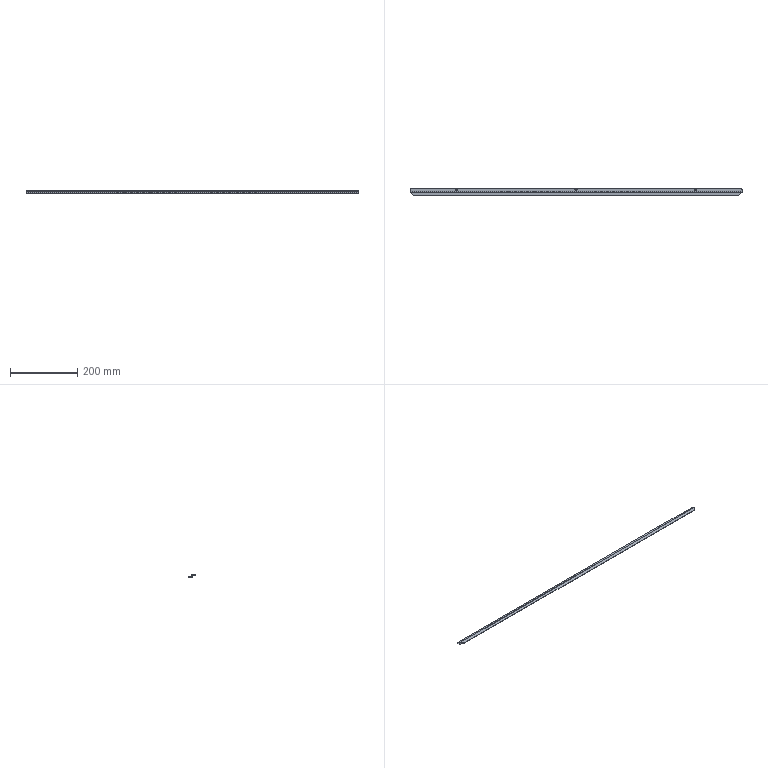Part | SolidWorks | features Chamfer 1, Fillet 1, FlatPattern 1, HoleWzd 1, SMBaseFlange 1, SheetMetal 1 | 1 solid | 30 faces | box 986 x 22 x 8.2 mm | volume 33274 mm3 | plane 18 | cylinder 12 | commonest cylinder face diameters 6 x8 0.4 x2 2.8 x2
STEP:
#1=CARTESIAN_POINT('',(-350.5,-5.,0.));
#2=VERTEX_POINT('',#1);
#3=CARTESIAN_POINT('',(-356.5,-5.,0.));
#4=VERTEX_POINT('',#3);
#5=CARTESIAN_POINT('',(-353.5,-5.,0.));
#6=DIRECTION('',(0.,0.,-1.));
#7=DIRECTION('',(0.,1.,0.));
#8=AXIS2_PLACEMENT_3D('',#5,#6,#7);
#9=CIRCLE('',#8,3.);
#10=EDGE_CURVE('',#2,#4,#9,.T.);
#11=ORIENTED_EDGE('',*,*,#10,.T.);
#12=CARTESIAN_POINT('',(-356.5,-5.,1.2));
#13=VERTEX_POINT('',#12);
#14=CARTESIAN_POINT('',(-356.5,-5.,1.2));
#15=DIRECTION('',(0.,0.,1.));
#16=VECTOR('',#15,1000.);
#17=LINE('',#14,#16);
#18=EDGE_CURVE('',#4,#13,#17,.T.);
#19=ORIENTED_EDGE('',*,*,#18,.T.);
#20=CARTESIAN_POINT('',(-350.5,-5.,1.2));
#21=VERTEX_POINT('',#20);
#22=CARTESIAN_POINT('',(-353.5,-5.,1.2));
#23=DIRECTION('',(0.,0.,1.));
#24=DIRECTION('',(1.,0.,0.));
#25=AXIS2_PLACEMENT_3D('',#22,#23,#24);
#26=CIRCLE('',#25,3.);
#27=EDGE_CURVE('',#13,#21,#26,.T.);
#28=ORIENTED_EDGE('',*,*,#27,.T.);
#29=CARTESIAN_POINT('',(-350.5,-5.,1.2));
#30=DIRECTION('',(0.,0.,1.));
#31=VECTOR('',#30,1000.);
#32=LINE('',#29,#31);
#33=EDGE_CURVE('',#2,#21,#32,.T.);
#34=ORIENTED_EDGE('',*,*,#33,.F.);
#35=EDGE_LOOP('',(#11,#19,#28,#34));
#36=FACE_OUTER_BOUND('',#35,.T.);
#37=CARTESIAN_POINT('',(-353.5,-5.,1.2));
#38=DIRECTION('',(0.,0.,1.));
#39=DIRECTION('',(1.,0.,0.));
#40=AXIS2_PLACEMENT_3D('',#37,#38,#39);
#41=CYLINDRICAL_SURFACE('',#40,3.);
#42=ADVANCED_FACE('',(#36),#41,.F.);
#43=CARTESIAN_POINT('',(3.,-5.,0.));
#44=VERTEX_POINT('',#43);
#45=CARTESIAN_POINT('',(-3.,-5.,0.));
#46=VERTEX_POINT('',#45);
#47=CARTESIAN_POINT('',(0.,-5.,0.));
#48=DIRECTION('',(0.,0.,-1.));
#49=DIRECTION('',(0.,1.,0.));
#50=AXIS2_PLACEMENT_3D('',#47,#48,#49);
#51=CIRCLE('',#50,3.);
#52=EDGE_CURVE('',#44,#46,#51,.T.);
#53=ORIENTED_EDGE('',*,*,#52,.T.);
#54=CARTESIAN_POINT('',(-3.,-5.,1.2));
#55=VERTEX_POINT('',#54);
#56=CARTESIAN_POINT('',(-3.,-5.,1.2));
#57=DIRECTION('',(0.,0.,1.));
#58=VECTOR('',#57,1000.);
#59=LINE('',#56,#58);
#60=EDGE_CURVE('',#46,#55,#59,.T.);
#61=ORIENTED_EDGE('',*,*,#60,.T.);
#62=CARTESIAN_POINT('',(3.,-5.,1.2));
#63=VERTEX_POINT('',#62);
#64=CARTESIAN_POINT('',(0.,-5.,1.2));
#65=DIRECTION('',(0.,0.,1.));
#66=DIRECTION('',(1.,0.,0.));
#67=AXIS2_PLACEMENT_3D('',#64,#65,#66);
#68=CIRCLE('',#67,3.);
#69=EDGE_CURVE('',#55,#63,#68,.T.);
#70=ORIENTED_EDGE('',*,*,#69,.T.);
#71=CARTESIAN_POINT('',(3.,-5.,1.2));
#72=DIRECTION('',(0.,0.,1.));
#73=VECTOR('',#72,1000.);
#74=LINE('',#71,#73);
#75=EDGE_CURVE('',#44,#63,#74,.T.);
#76=ORIENTED_EDGE('',*,*,#75,.F.);
#77=EDGE_LOOP('',(#53,#61,#70,#76));
#78=FACE_OUTER_BOUND('',#77,.T.);
#79=CARTESIAN_POINT('',(0.,-5.,1.2));
#80=DIRECTION('',(0.,0.,1.));
#81=DIRECTION('',(1.,0.,0.));
#82=AXIS2_PLACEMENT_3D('',#79,#80,#81);
#83=CYLINDRICAL_SURFACE('',#82,3.);
#84=ADVANCED_FACE('',(#78),#83,.F.);
#85=CARTESIAN_POINT('',(356.5,-5.,0.));
#86=VERTEX_POINT('',#85);
#87=CARTESIAN_POINT('',(350.5,-5.,0.));
#88=VERTEX_POINT('',#87);
#89=CARTESIAN_POINT('',(353.5,-5.,0.));
#90=DIRECTION('',(0.,0.,-1.));
#91=DIRECTION('',(0.,1.,0.));
#92=AXIS2_PLACEMENT_3D('',#89,#90,#91);
#93=CIRCLE('',#92,3.);
#94=EDGE_CURVE('',#86,#88,#93,.T.);
#95=ORIENTED_EDGE('',*,*,#94,.T.);
#96=CARTESIAN_POINT('',(350.5,-5.,1.2));
#97=VERTEX_POINT('',#96);
#98=CARTESIAN_POINT('',(350.5,-5.,1.2));
#99=DIRECTION('',(0.,0.,1.));
#100=VECTOR('',#99,1000.);
#101=LINE('',#98,#100);
#102=EDGE_CURVE('',#88,#97,#101,.T.);
#103=ORIENTED_EDGE('',*,*,#102,.T.);
#104=CARTESIAN_POINT('',(356.5,-5.,1.2));
#105=VERTEX_POINT('',#104);
#106=CARTESIAN_POINT('',(353.5,-5.,1.2));
#107=DIRECTION('',(0.,0.,1.));
#108=DIRECTION('',(1.,0.,0.));
#109=AXIS2_PLACEMENT_3D('',#106,#107,#108);
#110=CIRCLE('',#109,3.);
#111=EDGE_CURVE('',#97,#105,#110,.T.);
#112=ORIENTED_EDGE('',*,*,#111,.T.);
#113=CARTESIAN_POINT('',(356.5,-5.,1.2));
#114=DIRECTION('',(0.,0.,1.));
#115=VECTOR('',#114,1000.);
#116=LINE('',#113,#115);
#117=EDGE_CURVE('',#86,#105,#116,.T.);
#118=ORIENTED_EDGE('',*,*,#117,.F.);
#119=EDGE_LOOP('',(#95,#103,#112,#118));
#120=FACE_OUTER_BOUND('',#119,.T.);
#121=CARTESIAN_POINT('',(353.5,-5.,1.2));
#122=DIRECTION('',(0.,0.,1.));
#123=DIRECTION('',(1.,0.,0.));
#124=AXIS2_PLACEMENT_3D('',#121,#122,#123);
#125=CYLINDRICAL_SURFACE('',#124,3.);
#126=ADVANCED_FACE('',(#120),#125,.F.);
#127=CARTESIAN_POINT('',(-353.5,-5.,1.2));
#128=DIRECTION('',(0.,0.,1.));
#129=DIRECTION('',(1.,0.,0.));
#130=AXIS2_PLACEMENT_3D('',#127,#128,#129);
#131=CIRCLE('',#130,3.);
#132=EDGE_CURVE('',#21,#13,#131,.T.);
#133=ORIENTED_EDGE('',*,*,#132,.F.);
#134=ORIENTED_EDGE('',*,*,#27,.F.);
#135=EDGE_LOOP('',(#133,#134));
#136=FACE_BOUND('',#135,.T.);
#137=CARTESIAN_POINT('',(353.5,-5.,1.2));
#138=DIRECTION('',(0.,0.,1.));
#139=DIRECTION('',(1.,0.,0.));
#140=AXIS2_PLACEMENT_3D('',#137,#138,#139);
#141=CIRCLE('',#140,3.);
#142=EDGE_CURVE('',#105,#97,#141,.T.);
#143=ORIENTED_EDGE('',*,*,#142,.F.);
#144=ORIENTED_EDGE('',*,*,#111,.F.);
#145=EDGE_LOOP('',(#143,#144));
#146=FACE_BOUND('',#145,.T.);
#147=CARTESIAN_POINT('',(490.,0.,1.2));
#148=VERTEX_POINT('',#147);
#149=CARTESIAN_POINT('',(-490.,0.,1.2));
#150=VERTEX_POINT('',#149);
#151=CARTESIAN_POINT('',(493.,0.,1.2));
#152=DIRECTION('',(-1.,0.,0.));
#153=VECTOR('',#152,1000.);
#154=LINE('',#151,#153);
#155=EDGE_CURVE('',#148,#150,#154,.T.);
#156=ORIENTED_EDGE('',*,*,#155,.T.);
#157=CARTESIAN_POINT('',(-493.,-3.,1.2));
#158=VERTEX_POINT('',#157);
#159=CARTESIAN_POINT('',(-490.,-3.,1.2));
#160=DIRECTION('',(0.,0.,1.));
#161=DIRECTION('',(0.,1.,0.));
#162=AXIS2_PLACEMENT_3D('',#159,#160,#161);
#163=CIRCLE('',#162,3.);
#164=EDGE_CURVE('',#150,#158,#163,.T.);
#165=ORIENTED_EDGE('',*,*,#164,.T.);
#166=CARTESIAN_POINT('',(-493.,-10.6,1.2));
#167=VERTEX_POINT('',#166);
#168=CARTESIAN_POINT('',(-493.,0.,1.2));
#169=DIRECTION('',(0.,-1.,0.));
#170=VECTOR('',#169,1000.);
#171=LINE('',#168,#170);
#172=EDGE_CURVE('',#158,#167,#171,.T.);
#173=ORIENTED_EDGE('',*,*,#172,.T.);
#174=CARTESIAN_POINT('',(493.,-10.6,1.2));
#175=VERTEX_POINT('',#174);
#176=CARTESIAN_POINT('',(493.,-10.6,1.2));
#177=DIRECTION('',(-1.,0.,0.));
#178=VECTOR('',#177,1000.);
#179=LINE('',#176,#178);
#180=EDGE_CURVE('',#175,#167,#179,.T.);
#181=ORIENTED_EDGE('',*,*,#180,.F.);
#182=CARTESIAN_POINT('',(493.,-3.,1.2));
#183=VERTEX_POINT('',#182);
#184=CARTESIAN_POINT('',(493.,0.,1.2));
#185=DIRECTION('',(0.,-1.,0.));
#186=VECTOR('',#185,1000.);
#187=LINE('',#184,#186);
#188=EDGE_CURVE('',#183,#175,#187,.T.);
#189=ORIENTED_EDGE('',*,*,#188,.F.);
#190=CARTESIAN_POINT('',(490.,-3.,1.2));
#191=DIRECTION('',(0.,0.,1.));
#192=DIRECTION('',(0.,1.,0.));
#193=AXIS2_PLACEMENT_3D('',#190,#191,#192);
#194=CIRCLE('',#193,3.);
#195=EDGE_CURVE('',#183,#148,#194,.T.);
#196=ORIENTED_EDGE('',*,*,#195,.T.);
#197=EDGE_LOOP('',(#156,#165,#173,#181,#189,#196));
#198=FACE_OUTER_BOUND('',#197,.T.);
#199=CARTESIAN_POINT('',(0.,-5.,1.2));
#200=DIRECTION('',(0.,0.,1.));
#201=DIRECTION('',(1.,0.,0.));
#202=AXIS2_PLACEMENT_3D('',#199,#200,#201);
#203=CIRCLE('',#202,3.);
#204=EDGE_CURVE('',#63,#55,#203,.T.);
#205=ORIENTED_EDGE('',*,*,#204,.F.);
#206=ORIENTED_EDGE('',*,*,#69,.F.);
#207=EDGE_LOOP('',(#205,#206));
#208=FACE_BOUND('',#207,.T.);
#209=CARTESIAN_POINT('',(493.,0.,1.2));
#210=DIRECTION('',(0.,0.,-1.));
#211=DIRECTION('',(0.,1.,0.));
#212=AXIS2_PLACEMENT_3D('',#209,#210,#211);
#213=PLANE('',#212);
#214=ADVANCED_FACE('',(#136,#146,#198,#208),#213,.F.);
#215=CARTESIAN_POINT('',(493.,-12.,1.4));
#216=VERTEX_POINT('',#215);
#217=CARTESIAN_POINT('',(493.,-10.8,1.4));
#218=VERTEX_POINT('',#217);
#219=CARTESIAN_POINT('',(493.,-12.,1.4));
#220=DIRECTION('',(0.,1.,0.));
#221=VECTOR('',#220,1000.);
#222=LINE('',#219,#221);
#223=EDGE_CURVE('',#216,#218,#222,.T.);
#224=ORIENTED_EDGE('',*,*,#223,.F.);
#225=CARTESIAN_POINT('',(493.,-10.6,0.));
#226=VERTEX_POINT('',#225);
#227=CARTESIAN_POINT('',(493.,-10.6,1.4));
#228=DIRECTION('',(-1.,0.,0.));
#229=DIRECTION('',(0.,0.,-1.));
#230=AXIS2_PLACEMENT_3D('',#227,#228,#229);
#231=CIRCLE('',#230,1.4);
#232=EDGE_CURVE('',#226,#216,#231,.T.);
#233=ORIENTED_EDGE('',*,*,#232,.F.);
#234=CARTESIAN_POINT('',(493.,-10.6,1.2));
#235=DIRECTION('',(0.,0.,-1.));
#236=VECTOR('',#235,1000.);
#237=LINE('',#234,#236);
#238=EDGE_CURVE('',#175,#226,#237,.T.);
#239=ORIENTED_EDGE('',*,*,#238,.F.);
#240=CARTESIAN_POINT('',(493.,-10.6,1.4));
#241=DIRECTION('',(-1.,0.,0.));
#242=DIRECTION('',(0.,0.,-1.));
#243=AXIS2_PLACEMENT_3D('',#240,#241,#242);
#244=CIRCLE('',#243,0.2);
#245=EDGE_CURVE('',#175,#218,#244,.T.);
#246=ORIENTED_EDGE('',*,*,#245,.T.);
#247=EDGE_LOOP('',(#224,#233,#239,#246));
#248=FACE_OUTER_BOUND('',#247,.T.);
#249=CARTESIAN_POINT('',(493.,-12.,1.4));
#250=DIRECTION('',(1.,0.,0.));
#251=DIRECTION('',(0.,0.,-1.));
#252=AXIS2_PLACEMENT_3D('',#249,#250,#251);
#253=PLANE('',#252);
#254=ADVANCED_FACE('',(#248),#253,.T.);
#255=CARTESIAN_POINT('',(493.,-12.,6.8));
#256=VERTEX_POINT('',#255);
#257=CARTESIAN_POINT('',(493.,-12.,0.));
#258=DIRECTION('',(0.,0.,1.));
#259=VECTOR('',#258,1000.);
#260=LINE('',#257,#259);
#261=EDGE_CURVE('',#216,#256,#260,.T.);
#262=ORIENTED_EDGE('',*,*,#261,.F.);
#263=ORIENTED_EDGE('',*,*,#223,.T.);
#264=CARTESIAN_POINT('',(493.,-10.8,6.8));
#265=VERTEX_POINT('',#264);
#266=CARTESIAN_POINT('',(493.,-10.8,0.));
#267=DIRECTION('',(0.,0.,1.));
#268=VECTOR('',#267,1000.);
#269=LINE('',#266,#268);
#270=EDGE_CURVE('',#218,#265,#269,.T.);
#271=ORIENTED_EDGE('',*,*,#270,.T.);
#272=CARTESIAN_POINT('',(493.,-10.8,6.8));
#273=DIRECTION('',(0.,-1.,0.));
#274=VECTOR('',#273,1000.);
#275=LINE('',#272,#274);
#276=EDGE_CURVE('',#265,#256,#275,.T.);
#277=ORIENTED_EDGE('',*,*,#276,.T.);
#278=EDGE_LOOP('',(#262,#263,#271,#277));
#279=FACE_OUTER_BOUND('',#278,.T.);
#280=CARTESIAN_POINT('',(493.,-10.6,1.2));
#281=DIRECTION('',(1.,0.,0.));
#282=DIRECTION('',(0.,0.,-1.));
#283=AXIS2_PLACEMENT_3D('',#280,#281,#282);
#284=PLANE('',#283);
#285=ADVANCED_FACE('',(#279),#284,.T.);
#286=CARTESIAN_POINT('',(-493.,-10.6,0.));
#287=VERTEX_POINT('',#286);
#288=CARTESIAN_POINT('',(-493.,-10.6,0.));
#289=DIRECTION('',(0.,0.,1.));
#290=VECTOR('',#289,1000.);
#291=LINE('',#288,#290);
#292=EDGE_CURVE('',#287,#167,#291,.T.);
#293=ORIENTED_EDGE('',*,*,#292,.F.);
#294=CARTESIAN_POINT('',(-493.,-12.,1.4));
#295=VERTEX_POINT('',#294);
#296=CARTESIAN_POINT('',(-493.,-10.6,1.4));
#297=DIRECTION('',(-1.,0.,0.));
#298=DIRECTION('',(0.,0.,-1.));
#299=AXIS2_PLACEMENT_3D('',#296,#297,#298);
#300=CIRCLE('',#299,1.4);
#301=EDGE_CURVE('',#287,#295,#300,.T.);
#302=ORIENTED_EDGE('',*,*,#301,.T.);
#303=CARTESIAN_POINT('',(-493.,-10.8,1.4));
#304=VERTEX_POINT('',#303);
#305=CARTESIAN_POINT('',(-493.,-10.8,1.4));
#306=DIRECTION('',(0.,-1.,0.));
#307=VECTOR('',#306,1000.);
#308=LINE('',#305,#307);
#309=EDGE_CURVE('',#304,#295,#308,.T.);
#310=ORIENTED_EDGE('',*,*,#309,.F.);
#311=CARTESIAN_POINT('',(-493.,-10.6,1.4));
#312=DIRECTION('',(-1.,0.,0.));
#313=DIRECTION('',(0.,0.,-1.));
#314=AXIS2_PLACEMENT_3D('',#311,#312,#313);
#315=CIRCLE('',#314,0.2);
#316=EDGE_CURVE('',#167,#304,#315,.T.);
#317=ORIENTED_EDGE('',*,*,#316,.F.);
#318=EDGE_LOOP('',(#293,#302,#310,#317));
#319=FACE_OUTER_BOUND('',#318,.T.);
#320=CARTESIAN_POINT('',(-493.,-10.6,0.));
#321=DIRECTION('',(-1.,0.,0.));
#322=DIRECTION('',(0.,0.,1.));
#323=AXIS2_PLACEMENT_3D('',#320,#321,#322);
#324=PLANE('',#323);
#325=ADVANCED_FACE('',(#319),#324,.T.);
#326=ORIENTED_EDGE('',*,*,#172,.F.);
#327=CARTESIAN_POINT('',(-493.,-3.,0.));
#328=VERTEX_POINT('',#327);
#329=CARTESIAN_POINT('',(-493.,-3.,1.4));
#330=DIRECTION('',(0.,0.,-1.));
#331=VECTOR('',#330,1000.);
#332=LINE('',#329,#331);
#333=EDGE_CURVE('',#158,#328,#332,.T.);
#334=ORIENTED_EDGE('',*,*,#333,.T.);
#335=CARTESIAN_POINT('',(-493.,0.,0.));
#336=DIRECTION('',(0.,-1.,0.));
#337=VECTOR('',#336,1000.);
#338=LINE('',#335,#337);
#339=EDGE_CURVE('',#328,#287,#338,.T.);
#340=ORIENTED_EDGE('',*,*,#339,.T.);
#341=ORIENTED_EDGE('',*,*,#292,.T.);
#342=EDGE_LOOP('',(#326,#334,#340,#341));
#343=FACE_OUTER_BOUND('',#342,.T.);
#344=CARTESIAN_POINT('',(-493.,-10.8,1.4));
#345=DIRECTION('',(-1.,0.,0.));
#346=DIRECTION('',(0.,0.,1.));
#347=AXIS2_PLACEMENT_3D('',#344,#345,#346);
#348=PLANE('',#347);
#349=ADVANCED_FACE('',(#343),#348,.T.);
#350=CARTESIAN_POINT('',(493.,-12.,8.186));
#351=VERTEX_POINT('',#350);
#352=CARTESIAN_POINT('',(493.,-12.2,6.8));
#353=DIRECTION('',(1.,0.,0.));
#354=DIRECTION('',(0.,0.,-1.));
#355=AXIS2_PLACEMENT_3D('',#352,#353,#354);
#356=CIRCLE('',#355,1.4);
#357=EDGE_CURVE('',#265,#351,#356,.T.);
#358=ORIENTED_EDGE('',*,*,#357,.T.);
#359=CARTESIAN_POINT('',(493.,-12.,7.));
#360=DIRECTION('',(0.,0.,-1.));
#361=VECTOR('',#360,1000.);
#362=LINE('',#359,#361);
#363=EDGE_CURVE('',#351,#256,#362,.T.);
#364=ORIENTED_EDGE('',*,*,#363,.T.);
#365=ORIENTED_EDGE('',*,*,#276,.F.);
#366=EDGE_LOOP('',(#358,#364,#365));
#367=FACE_OUTER_BOUND('',#366,.T.);
#368=CARTESIAN_POINT('',(493.,-12.2,7.));
#369=DIRECTION('',(1.,0.,0.));
#370=DIRECTION('',(0.,0.,-1.));
#371=AXIS2_PLACEMENT_3D('',#368,#369,#370);
#372=PLANE('',#371);
#373=ADVANCED_FACE('',(#367),#372,.T.);
#374=CARTESIAN_POINT('',(-493.,-12.,6.8));
#375=VERTEX_POINT('',#374);
#376=CARTESIAN_POINT('',(-493.,-10.8,6.8));
#377=VERTEX_POINT('',#376);
#378=CARTESIAN_POINT('',(-493.,-12.,6.8));
#379=DIRECTION('',(0.,1.,0.));
#380=VECTOR('',#379,1000.);
#381=LINE('',#378,#380);
#382=EDGE_CURVE('',#375,#377,#381,.T.);
#383=ORIENTED_EDGE('',*,*,#382,.F.);
#384=CARTESIAN_POINT('',(-493.,-12.,8.186));
#385=VERTEX_POINT('',#384);
#386=CARTESIAN_POINT('',(-493.,-12.,6.8));
#387=DIRECTION('',(0.,0.,1.));
#388=VECTOR('',#387,1000.);
#389=LINE('',#386,#388);
#390=EDGE_CURVE('',#375,#385,#389,.T.);
#391=ORIENTED_EDGE('',*,*,#390,.T.);
#392=CARTESIAN_POINT('',(-493.,-12.2,6.8));
#393=DIRECTION('',(1.,0.,0.));
#394=DIRECTION('',(0.,0.,-1.));
#395=AXIS2_PLACEMENT_3D('',#392,#393,#394);
#396=CIRCLE('',#395,1.4);
#397=EDGE_CURVE('',#377,#385,#396,.T.);
#398=ORIENTED_EDGE('',*,*,#397,.F.);
#399=EDGE_LOOP('',(#383,#391,#398));
#400=FACE_OUTER_BOUND('',#399,.T.);
#401=CARTESIAN_POINT('',(-493.,-12.,6.8));
#402=DIRECTION('',(-1.,0.,0.));
#403=DIRECTION('',(0.,0.,1.));
#404=AXIS2_PLACEMENT_3D('',#401,#402,#403);
#405=PLANE('',#404);
#406=ADVANCED_FACE('',(#400),#405,.T.);
#407=CARTESIAN_POINT('',(-493.,-12.,0.));
#408=DIRECTION('',(0.,0.,1.));
#409=VECTOR('',#408,1000.);
#410=LINE('',#407,#409);
#411=EDGE_CURVE('',#295,#375,#410,.T.);
#412=ORIENTED_EDGE('',*,*,#411,.T.);
#413=ORIENTED_EDGE('',*,*,#382,.T.);
#414=CARTESIAN_POINT('',(-493.,-10.8,0.));
#415=DIRECTION('',(0.,0.,1.));
#416=VECTOR('',#415,1000.);
#417=LINE('',#414,#416);
#418=EDGE_CURVE('',#304,#377,#417,.T.);
#419=ORIENTED_EDGE('',*,*,#418,.F.);
#420=ORIENTED_EDGE('',*,*,#309,.T.);
#421=EDGE_LOOP('',(#412,#413,#419,#420));
#422=FACE_OUTER_BOUND('',#421,.T.);
#423=CARTESIAN_POINT('',(-493.,-12.2,8.2));
#424=DIRECTION('',(-1.,0.,0.));
#425=DIRECTION('',(0.,0.,1.));
#426=AXIS2_PLACEMENT_3D('',#423,#424,#425);
#427=PLANE('',#426);
#428=ADVANCED_FACE('',(#422),#427,.T.);
#429=CARTESIAN_POINT('',(483.,-22.,8.2));
#430=VERTEX_POINT('',#429);
#431=CARTESIAN_POINT('',(-483.,-22.,8.2));
#432=VERTEX_POINT('',#431);
#433=CARTESIAN_POINT('',(493.,-22.,8.2));
#434=DIRECTION('',(-1.,0.,0.));
#435=VECTOR('',#434,1000.);
#436=LINE('',#433,#435);
#437=EDGE_CURVE('',#430,#432,#436,.T.);
#438=ORIENTED_EDGE('',*,*,#437,.F.);
#439=CARTESIAN_POINT('',(492.8,-12.2,8.2));
#440=VERTEX_POINT('',#439);
#441=CARTESIAN_POINT('',(483.,-22.,8.2));
#442=DIRECTION('',(0.7071,0.7071,0.));
#443=VECTOR('',#442,1000.);
#444=LINE('',#441,#443);
#445=EDGE_CURVE('',#430,#440,#444,.T.);
#446=ORIENTED_EDGE('',*,*,#445,.T.);
#447=CARTESIAN_POINT('',(-492.8,-12.2,8.2));
#448=VERTEX_POINT('',#447);
#449=CARTESIAN_POINT('',(493.,-12.2,8.2));
#450=DIRECTION('',(-1.,0.,0.));
#451=VECTOR('',#450,1000.);
#452=LINE('',#449,#451);
#453=EDGE_CURVE('',#440,#448,#452,.T.);
#454=ORIENTED_EDGE('',*,*,#453,.T.);
#455=CARTESIAN_POINT('',(-493.,-12.,8.2));
#456=DIRECTION('',(0.7071,-0.7071,0.));
#457=VECTOR('',#456,1000.);
#458=LINE('',#455,#457);
#459=EDGE_CURVE('',#448,#432,#458,.T.);
#460=ORIENTED_EDGE('',*,*,#459,.T.);
#461=EDGE_LOOP('',(#438,#446,#454,#460));
#462=FACE_OUTER_BOUND('',#461,.T.);
#463=CARTESIAN_POINT('',(493.,-12.,8.2));
#464=DIRECTION('',(0.,0.,-1.));
#465=DIRECTION('',(0.,1.,0.));
#466=AXIS2_PLACEMENT_3D('',#463,#464,#465);
#467=PLANE('',#466);
#468=ADVANCED_FACE('',(#462),#467,.F.);
#469=CARTESIAN_POINT('',(483.,-22.,7.));
#470=VERTEX_POINT('',#469);
#471=CARTESIAN_POINT('',(-483.,-22.,7.));
#472=VERTEX_POINT('',#471);
#473=CARTESIAN_POINT('',(493.,-22.,7.));
#474=DIRECTION('',(-1.,0.,0.));
#475=VECTOR('',#474,1000.);
#476=LINE('',#473,#475);
#477=EDGE_CURVE('',#470,#472,#476,.T.);
#478=ORIENTED_EDGE('',*,*,#477,.F.);
#479=CARTESIAN_POINT('',(483.,-22.,7.));
#480=DIRECTION('',(0.,0.,1.));
#481=VECTOR('',#480,1000.);
#482=LINE('',#479,#481);
#483=EDGE_CURVE('',#470,#430,#482,.T.);
#484=ORIENTED_EDGE('',*,*,#483,.T.);
#485=ORIENTED_EDGE('',*,*,#437,.T.);
#486=CARTESIAN_POINT('',(-483.,-22.,7.));
#487=DIRECTION('',(0.,0.,-1.));
#488=VECTOR('',#487,1000.);
#489=LINE('',#486,#488);
#490=EDGE_CURVE('',#432,#472,#489,.T.);
#491=ORIENTED_EDGE('',*,*,#490,.T.);
#492=EDGE_LOOP('',(#478,#484,#485,#491));
#493=FACE_OUTER_BOUND('',#492,.T.);
#494=CARTESIAN_POINT('',(493.,-22.,7.));
#495=DIRECTION('',(0.,-1.,0.));
#496=DIRECTION('',(0.,0.,-1.));
#497=AXIS2_PLACEMENT_3D('',#494,#495,#496);
#498=PLANE('',#497);
#499=ADVANCED_FACE('',(#493),#498,.T.);
#500=CARTESIAN_POINT('',(492.8,-12.2,7.));
#501=VERTEX_POINT('',#500);
#502=CARTESIAN_POINT('',(-492.8,-12.2,7.));
#503=VERTEX_POINT('',#502);
#504=CARTESIAN_POINT('',(493.,-12.2,7.));
#505=DIRECTION('',(-1.,0.,0.));
#506=VECTOR('',#505,1000.);
#507=LINE('',#504,#506);
#508=EDGE_CURVE('',#501,#503,#507,.T.);
#509=ORIENTED_EDGE('',*,*,#508,.F.);
#510=CARTESIAN_POINT('',(493.,-12.,7.));
#511=DIRECTION('',(-0.7071,-0.7071,0.));
#512=VECTOR('',#511,1000.);
#513=LINE('',#510,#512);
#514=EDGE_CURVE('',#501,#470,#513,.T.);
#515=ORIENTED_EDGE('',*,*,#514,.T.);
#516=ORIENTED_EDGE('',*,*,#477,.T.);
#517=CARTESIAN_POINT('',(0.,-505.,7.));
#518=DIRECTION('',(-0.7071,0.7071,0.));
#519=VECTOR('',#518,1000.);
#520=LINE('',#517,#519);
#521=EDGE_CURVE('',#472,#503,#520,.T.);
#522=ORIENTED_EDGE('',*,*,#521,.T.);
#523=EDGE_LOOP('',(#509,#515,#516,#522));
#524=FACE_OUTER_BOUND('',#523,.T.);
#525=CARTESIAN_POINT('',(493.,-12.,7.));
#526=DIRECTION('',(0.,0.,-1.));
#527=DIRECTION('',(0.,1.,0.));
#528=AXIS2_PLACEMENT_3D('',#525,#526,#527);
#529=PLANE('',#528);
#530=ADVANCED_FACE('',(#524),#529,.T.);
#531=CARTESIAN_POINT('',(493.,-12.,6.8));
#532=DIRECTION('',(-1.,0.,0.));
#533=VECTOR('',#532,1000.);
#534=LINE('',#531,#533);
#535=EDGE_CURVE('',#256,#375,#534,.T.);
#536=ORIENTED_EDGE('',*,*,#535,.F.);
#537=CARTESIAN_POINT('',(493.,-12.,6.8));
#538=CARTESIAN_POINT('',(493.,-12.,6.917));
#539=CARTESIAN_POINT('',(492.917,-12.083,7.));
#540=CARTESIAN_POINT('',(492.8,-12.2,7.));
#541=(BOUNDED_CURVE()B_SPLINE_CURVE(3,(#537,#538,#539,#540),.UNSPECIFIED.,.F.,.F.)B_SPLINE_CURVE_WITH_KNOTS((4,4),(3.142,4.712),.UNSPECIFIED.)CURVE()GEOMETRIC_REPRESENTATION_ITEM()RATIONAL_B_SPLINE_CURVE((1.,0.8047,0.8047,1.))REPRESENTATION_ITEM(''));
#542=EDGE_CURVE('',#256,#501,#541,.T.);
#543=ORIENTED_EDGE('',*,*,#542,.T.);
#544=ORIENTED_EDGE('',*,*,#508,.T.);
#545=CARTESIAN_POINT('',(-492.8,-12.2,7.));
#546=CARTESIAN_POINT('',(-492.917,-12.083,7.));
#547=CARTESIAN_POINT('',(-493.,-12.,6.917));
#548=CARTESIAN_POINT('',(-493.,-12.,6.8));
#549=(BOUNDED_CURVE()B_SPLINE_CURVE(3,(#545,#546,#547,#548),.UNSPECIFIED.,.F.,.F.)B_SPLINE_CURVE_WITH_KNOTS((4,4),(4.712,6.283),.UNSPECIFIED.)CURVE()GEOMETRIC_REPRESENTATION_ITEM()RATIONAL_B_SPLINE_CURVE((1.,0.8047,0.8047,1.))REPRESENTATION_ITEM(''));
#550=EDGE_CURVE('',#503,#375,#549,.T.);
#551=ORIENTED_EDGE('',*,*,#550,.T.);
#552=EDGE_LOOP('',(#536,#543,#544,#551));
#553=FACE_OUTER_BOUND('',#552,.T.);
#554=CARTESIAN_POINT('',(493.,-12.2,6.8));
#555=DIRECTION('',(-1.,0.,0.));
#556=DIRECTION('',(0.,0.,1.));
#557=AXIS2_PLACEMENT_3D('',#554,#555,#556);
#558=CYLINDRICAL_SURFACE('',#557,0.2);
#559=ADVANCED_FACE('',(#553),#558,.F.);
#560=ORIENTED_EDGE('',*,*,#411,.F.);
#561=CARTESIAN_POINT('',(493.,-12.,1.4));
#562=DIRECTION('',(-1.,0.,0.));
#563=VECTOR('',#562,1000.);
#564=LINE('',#561,#563);
#565=EDGE_CURVE('',#216,#295,#564,.T.);
#566=ORIENTED_EDGE('',*,*,#565,.F.);
#567=ORIENTED_EDGE('',*,*,#261,.T.);
#568=ORIENTED_EDGE('',*,*,#535,.T.);
#569=EDGE_LOOP('',(#560,#566,#567,#568));
#570=FACE_OUTER_BOUND('',#569,.T.);
#571=CARTESIAN_POINT('',(493.,-12.,0.));
#572=DIRECTION('',(0.,-1.,0.));
#573=DIRECTION('',(0.,0.,-1.));
#574=AXIS2_PLACEMENT_3D('',#571,#572,#573);
#575=PLANE('',#574);
#576=ADVANCED_FACE('',(#570),#575,.T.);
#577=ORIENTED_EDGE('',*,*,#301,.F.);
#578=CARTESIAN_POINT('',(493.,-10.6,0.));
#579=DIRECTION('',(-1.,0.,0.));
#580=VECTOR('',#579,1000.);
#581=LINE('',#578,#580);
#582=EDGE_CURVE('',#226,#287,#581,.T.);
#583=ORIENTED_EDGE('',*,*,#582,.F.);
#584=ORIENTED_EDGE('',*,*,#232,.T.);
#585=ORIENTED_EDGE('',*,*,#565,.T.);
#586=EDGE_LOOP('',(#577,#583,#584,#585));
#587=FACE_OUTER_BOUND('',#586,.T.);
#588=CARTESIAN_POINT('',(493.,-10.6,1.4));
#589=DIRECTION('',(-1.,0.,0.));
#590=DIRECTION('',(0.,0.,1.));
#591=AXIS2_PLACEMENT_3D('',#588,#589,#590);
#592=CYLINDRICAL_SURFACE('',#591,1.4);
#593=ADVANCED_FACE('',(#587),#592,.T.);
#594=ORIENTED_EDGE('',*,*,#10,.F.);
#595=CARTESIAN_POINT('',(-353.5,-5.,0.));
#596=DIRECTION('',(0.,0.,-1.));
#597=DIRECTION('',(0.,1.,0.));
#598=AXIS2_PLACEMENT_3D('',#595,#596,#597);
#599=CIRCLE('',#598,3.);
#600=EDGE_CURVE('',#4,#2,#599,.T.);
#601=ORIENTED_EDGE('',*,*,#600,.F.);
#602=EDGE_LOOP('',(#594,#601));
#603=FACE_BOUND('',#602,.T.);
#604=ORIENTED_EDGE('',*,*,#52,.F.);
#605=CARTESIAN_POINT('',(0.,-5.,0.));
#606=DIRECTION('',(0.,0.,-1.));
#607=DIRECTION('',(0.,1.,0.));
#608=AXIS2_PLACEMENT_3D('',#605,#606,#607);
#609=CIRCLE('',#608,3.);
#610=EDGE_CURVE('',#46,#44,#609,.T.);
#611=ORIENTED_EDGE('',*,*,#610,.F.);
#612=EDGE_LOOP('',(#604,#611));
#613=FACE_BOUND('',#612,.T.);
#614=ORIENTED_EDGE('',*,*,#94,.F.);
#615=CARTESIAN_POINT('',(353.5,-5.,0.));
#616=DIRECTION('',(0.,0.,-1.));
#617=DIRECTION('',(0.,1.,0.));
#618=AXIS2_PLACEMENT_3D('',#615,#616,#617);
#619=CIRCLE('',#618,3.);
#620=EDGE_CURVE('',#88,#86,#619,.T.);
#621=ORIENTED_EDGE('',*,*,#620,.F.);
#622=EDGE_LOOP('',(#614,#621));
#623=FACE_BOUND('',#622,.T.);
#624=ORIENTED_EDGE('',*,*,#339,.F.);
#625=CARTESIAN_POINT('',(-490.,0.,0.));
#626=VERTEX_POINT('',#625);
#627=CARTESIAN_POINT('',(-490.,-3.,0.));
#628=DIRECTION('',(0.,0.,-1.));
#629=DIRECTION('',(0.,1.,0.));
#630=AXIS2_PLACEMENT_3D('',#627,#628,#629);
#631=CIRCLE('',#630,3.);
#632=EDGE_CURVE('',#328,#626,#631,.T.);
#633=ORIENTED_EDGE('',*,*,#632,.T.);
#634=CARTESIAN_POINT('',(490.,0.,0.));
#635=VERTEX_POINT('',#634);
#636=CARTESIAN_POINT('',(493.,0.,0.));
#637=DIRECTION('',(-1.,0.,0.));
#638=VECTOR('',#637,1000.);
#639=LINE('',#636,#638);
#640=EDGE_CURVE('',#635,#626,#639,.T.);
#641=ORIENTED_EDGE('',*,*,#640,.F.);
#642=CARTESIAN_POINT('',(493.,-3.,0.));
#643=VERTEX_POINT('',#642);
#644=CARTESIAN_POINT('',(490.,-3.,0.));
#645=DIRECTION('',(0.,0.,-1.));
#646=DIRECTION('',(0.,1.,0.));
#647=AXIS2_PLACEMENT_3D('',#644,#645,#646);
#648=CIRCLE('',#647,3.);
#649=EDGE_CURVE('',#635,#643,#648,.T.);
#650=ORIENTED_EDGE('',*,*,#649,.T.);
#651=CARTESIAN_POINT('',(493.,0.,0.));
#652=DIRECTION('',(0.,-1.,0.));
#653=VECTOR('',#652,1000.);
#654=LINE('',#651,#653);
#655=EDGE_CURVE('',#643,#226,#654,.T.);
#656=ORIENTED_EDGE('',*,*,#655,.T.);
#657=ORIENTED_EDGE('',*,*,#582,.T.);
#658=EDGE_LOOP('',(#624,#633,#641,#650,#656,#657));
#659=FACE_OUTER_BOUND('',#658,.T.);
#660=CARTESIAN_POINT('',(493.,0.,0.));
#661=DIRECTION('',(0.,0.,-1.));
#662=DIRECTION('',(0.,1.,0.));
#663=AXIS2_PLACEMENT_3D('',#660,#661,#662);
#664=PLANE('',#663);
#665=ADVANCED_FACE('',(#603,#613,#623,#659),#664,.T.);
#666=ORIENTED_EDGE('',*,*,#640,.T.);
#667=CARTESIAN_POINT('',(-490.,0.,1.2));
#668=DIRECTION('',(0.,0.,1.));
#669=VECTOR('',#668,1000.);
#670=LINE('',#667,#669);
#671=EDGE_CURVE('',#626,#150,#670,.T.);
#672=ORIENTED_EDGE('',*,*,#671,.T.);
#673=ORIENTED_EDGE('',*,*,#155,.F.);
#674=CARTESIAN_POINT('',(490.,0.,0.));
#675=DIRECTION('',(0.,0.,-1.));
#676=VECTOR('',#675,1000.);
#677=LINE('',#674,#676);
#678=EDGE_CURVE('',#148,#635,#677,.T.);
#679=ORIENTED_EDGE('',*,*,#678,.T.);
#680=EDGE_LOOP('',(#666,#672,#673,#679));
#681=FACE_OUTER_BOUND('',#680,.T.);
#682=CARTESIAN_POINT('',(493.,0.,1.2));
#683=DIRECTION('',(0.,1.,0.));
#684=DIRECTION('',(0.,0.,1.));
#685=AXIS2_PLACEMENT_3D('',#682,#683,#684);
#686=PLANE('',#685);
#687=ADVANCED_FACE('',(#681),#686,.T.);
#688=ORIENTED_EDGE('',*,*,#316,.T.);
#689=CARTESIAN_POINT('',(493.,-10.8,1.4));
#690=DIRECTION('',(-1.,0.,0.));
#691=VECTOR('',#690,1000.);
#692=LINE('',#689,#691);
#693=EDGE_CURVE('',#218,#304,#692,.T.);
#694=ORIENTED_EDGE('',*,*,#693,.F.);
#695=ORIENTED_EDGE('',*,*,#245,.F.);
#696=ORIENTED_EDGE('',*,*,#180,.T.);
#697=EDGE_LOOP('',(#688,#694,#695,#696));
#698=FACE_OUTER_BOUND('',#697,.T.);
#699=CARTESIAN_POINT('',(493.,-10.6,1.4));
#700=DIRECTION('',(-1.,0.,0.));
#701=DIRECTION('',(0.,0.,1.));
#702=AXIS2_PLACEMENT_3D('',#699,#700,#701);
#703=CYLINDRICAL_SURFACE('',#702,0.2);
#704=ADVANCED_FACE('',(#698),#703,.F.);
#705=ORIENTED_EDGE('',*,*,#418,.T.);
#706=CARTESIAN_POINT('',(493.,-10.8,6.8));
#707=DIRECTION('',(-1.,0.,0.));
#708=VECTOR('',#707,1000.);
#709=LINE('',#706,#708);
#710=EDGE_CURVE('',#265,#377,#709,.T.);
#711=ORIENTED_EDGE('',*,*,#710,.F.);
#712=ORIENTED_EDGE('',*,*,#270,.F.);
#713=ORIENTED_EDGE('',*,*,#693,.T.);
#714=EDGE_LOOP('',(#705,#711,#712,#713));
#715=FACE_OUTER_BOUND('',#714,.T.);
#716=CARTESIAN_POINT('',(493.,-10.8,0.));
#717=DIRECTION('',(0.,-1.,0.));
#718=DIRECTION('',(0.,0.,-1.));
#719=AXIS2_PLACEMENT_3D('',#716,#717,#718);
#720=PLANE('',#719);
#721=ADVANCED_FACE('',(#715),#720,.F.);
#722=ORIENTED_EDGE('',*,*,#453,.F.);
#723=CARTESIAN_POINT('',(492.8,-12.2,8.2));
#724=CARTESIAN_POINT('',(492.867,-12.133,8.2));
#725=CARTESIAN_POINT('',(492.934,-12.066,8.195));
#726=CARTESIAN_POINT('',(493.,-12.,8.186));
#727=(BOUNDED_CURVE()B_SPLINE_CURVE(3,(#723,#724,#725,#726),.UNSPECIFIED.,.F.,.F.)B_SPLINE_CURVE_WITH_KNOTS((4,4),(1.571,1.714),.UNSPECIFIED.)CURVE()GEOMETRIC_REPRESENTATION_ITEM()RATIONAL_B_SPLINE_CURVE((1.,0.9983,0.9983,1.))REPRESENTATION_ITEM(''));
#728=EDGE_CURVE('',#440,#351,#727,.T.);
#729=ORIENTED_EDGE('',*,*,#728,.T.);
#730=ORIENTED_EDGE('',*,*,#357,.F.);
#731=ORIENTED_EDGE('',*,*,#710,.T.);
#732=ORIENTED_EDGE('',*,*,#397,.T.);
#733=CARTESIAN_POINT('',(-493.,-12.,8.186));
#734=CARTESIAN_POINT('',(-492.934,-12.066,8.195));
#735=CARTESIAN_POINT('',(-492.867,-12.133,8.2));
#736=CARTESIAN_POINT('',(-492.8,-12.2,8.2));
#737=(BOUNDED_CURVE()B_SPLINE_CURVE(3,(#733,#734,#735,#736),.UNSPECIFIED.,.F.,.F.)B_SPLINE_CURVE_WITH_KNOTS((4,4),(1.427,1.571),.UNSPECIFIED.)CURVE()GEOMETRIC_REPRESENTATION_ITEM()RATIONAL_B_SPLINE_CURVE((1.,0.9983,0.9983,1.))REPRESENTATION_ITEM(''));
#738=EDGE_CURVE('',#385,#448,#737,.T.);
#739=ORIENTED_EDGE('',*,*,#738,.T.);
#740=EDGE_LOOP('',(#722,#729,#730,#731,#732,#739));
#741=FACE_OUTER_BOUND('',#740,.T.);
#742=CARTESIAN_POINT('',(493.,-12.2,6.8));
#743=DIRECTION('',(-1.,0.,0.));
#744=DIRECTION('',(0.,0.,1.));
#745=AXIS2_PLACEMENT_3D('',#742,#743,#744);
#746=CYLINDRICAL_SURFACE('',#745,1.4);
#747=ADVANCED_FACE('',(#741),#746,.T.);
#748=ORIENTED_EDGE('',*,*,#655,.F.);
#749=CARTESIAN_POINT('',(493.,-3.,1.2));
#750=DIRECTION('',(0.,0.,1.));
#751=VECTOR('',#750,1000.);
#752=LINE('',#749,#751);
#753=EDGE_CURVE('',#643,#183,#752,.T.);
#754=ORIENTED_EDGE('',*,*,#753,.T.);
#755=ORIENTED_EDGE('',*,*,#188,.T.);
#756=ORIENTED_EDGE('',*,*,#238,.T.);
#757=EDGE_LOOP('',(#748,#754,#755,#756));
#758=FACE_OUTER_BOUND('',#757,.T.);
#759=CARTESIAN_POINT('',(493.,-12.2,6.8));
#760=DIRECTION('',(-1.,0.,0.));
#761=DIRECTION('',(0.,0.,1.));
#762=AXIS2_PLACEMENT_3D('',#759,#760,#761);
#763=PLANE('',#762);
#764=ADVANCED_FACE('',(#758),#763,.F.);
#765=ORIENTED_EDGE('',*,*,#102,.F.);
#766=ORIENTED_EDGE('',*,*,#620,.T.);
#767=ORIENTED_EDGE('',*,*,#117,.T.);
#768=ORIENTED_EDGE('',*,*,#142,.T.);
#769=EDGE_LOOP('',(#765,#766,#767,#768));
#770=FACE_OUTER_BOUND('',#769,.T.);
#771=CARTESIAN_POINT('',(353.5,-5.,1.2));
#772=DIRECTION('',(0.,0.,1.));
#773=DIRECTION('',(1.,0.,0.));
#774=AXIS2_PLACEMENT_3D('',#771,#772,#773);
#775=CYLINDRICAL_SURFACE('',#774,3.);
#776=ADVANCED_FACE('',(#770),#775,.F.);
#777=ORIENTED_EDGE('',*,*,#60,.F.);
#778=ORIENTED_EDGE('',*,*,#610,.T.);
#779=ORIENTED_EDGE('',*,*,#75,.T.);
#780=ORIENTED_EDGE('',*,*,#204,.T.);
#781=EDGE_LOOP('',(#777,#778,#779,#780));
#782=FACE_OUTER_BOUND('',#781,.T.);
#783=CARTESIAN_POINT('',(0.,-5.,1.2));
#784=DIRECTION('',(0.,0.,1.));
#785=DIRECTION('',(1.,0.,0.));
#786=AXIS2_PLACEMENT_3D('',#783,#784,#785);
#787=CYLINDRICAL_SURFACE('',#786,3.);
#788=ADVANCED_FACE('',(#782),#787,.F.);
#789=ORIENTED_EDGE('',*,*,#18,.F.);
#790=ORIENTED_EDGE('',*,*,#600,.T.);
#791=ORIENTED_EDGE('',*,*,#33,.T.);
#792=ORIENTED_EDGE('',*,*,#132,.T.);
#793=EDGE_LOOP('',(#789,#790,#791,#792));
#794=FACE_OUTER_BOUND('',#793,.T.);
#795=CARTESIAN_POINT('',(-353.5,-5.,1.2));
#796=DIRECTION('',(0.,0.,1.));
#797=DIRECTION('',(1.,0.,0.));
#798=AXIS2_PLACEMENT_3D('',#795,#796,#797);
#799=CYLINDRICAL_SURFACE('',#798,3.);
#800=ADVANCED_FACE('',(#794),#799,.F.);
#801=ORIENTED_EDGE('',*,*,#542,.F.);
#802=ORIENTED_EDGE('',*,*,#363,.F.);
#803=ORIENTED_EDGE('',*,*,#728,.F.);
#804=ORIENTED_EDGE('',*,*,#445,.F.);
#805=ORIENTED_EDGE('',*,*,#483,.F.);
#806=ORIENTED_EDGE('',*,*,#514,.F.);
#807=EDGE_LOOP('',(#801,#802,#803,#804,#805,#806));
#808=FACE_OUTER_BOUND('',#807,.T.);
#809=CARTESIAN_POINT('',(483.,-22.,7.));
#810=DIRECTION('',(-0.7071,0.7071,0.));
#811=DIRECTION('',(0.,0.,1.));
#812=AXIS2_PLACEMENT_3D('',#809,#810,#811);
#813=PLANE('',#812);
#814=ADVANCED_FACE('',(#808),#813,.F.);
#815=ORIENTED_EDGE('',*,*,#521,.F.);
#816=ORIENTED_EDGE('',*,*,#490,.F.);
#817=ORIENTED_EDGE('',*,*,#459,.F.);
#818=ORIENTED_EDGE('',*,*,#738,.F.);
#819=ORIENTED_EDGE('',*,*,#390,.F.);
#820=ORIENTED_EDGE('',*,*,#550,.F.);
#821=EDGE_LOOP('',(#815,#816,#817,#818,#819,#820));
#822=FACE_OUTER_BOUND('',#821,.T.);
#823=CARTESIAN_POINT('',(-493.,-12.,6.8));
#824=DIRECTION('',(0.7071,0.7071,0.));
#825=DIRECTION('',(0.,0.,1.));
#826=AXIS2_PLACEMENT_3D('',#823,#824,#825);
#827=PLANE('',#826);
#828=ADVANCED_FACE('',(#822),#827,.F.);
#829=ORIENTED_EDGE('',*,*,#164,.F.);
#830=ORIENTED_EDGE('',*,*,#671,.F.);
#831=ORIENTED_EDGE('',*,*,#632,.F.);
#832=ORIENTED_EDGE('',*,*,#333,.F.);
#833=EDGE_LOOP('',(#829,#830,#831,#832));
#834=FACE_OUTER_BOUND('',#833,.T.);
#835=CARTESIAN_POINT('',(-490.,-3.,1.4));
#836=DIRECTION('',(0.,0.,-1.));
#837=DIRECTION('',(0.,1.,0.));
#838=AXIS2_PLACEMENT_3D('',#835,#836,#837);
#839=CYLINDRICAL_SURFACE('',#838,3.);
#840=ADVANCED_FACE('',(#834),#839,.T.);
#841=ORIENTED_EDGE('',*,*,#195,.F.);
#842=ORIENTED_EDGE('',*,*,#753,.F.);
#843=ORIENTED_EDGE('',*,*,#649,.F.);
#844=ORIENTED_EDGE('',*,*,#678,.F.);
#845=EDGE_LOOP('',(#841,#842,#843,#844));
#846=FACE_OUTER_BOUND('',#845,.T.);
#847=CARTESIAN_POINT('',(490.,-3.,1.2));
#848=DIRECTION('',(0.,0.,1.));
#849=DIRECTION('',(0.,-1.,0.));
#850=AXIS2_PLACEMENT_3D('',#847,#848,#849);
#851=CYLINDRICAL_SURFACE('',#850,3.);
#852=ADVANCED_FACE('',(#846),#851,.T.);
#853=CLOSED_SHELL('',(#42,#84,#126,#214,#254,#285,#325,#349,#373,#406,#428,#468,#499,#530,#559,#576,#593,#665,#687,#704,#721,#747,#764,#776,#788,#800,#814,#828,#840,#852));
#854=MANIFOLD_SOLID_BREP('',#853);
#855=CARTESIAN_POINT('',(0.,0.,0.));
#856=DIRECTION('',(0.,0.,1.));
#857=DIRECTION('',(1.,0.,0.));
#858=AXIS2_PLACEMENT_3D('',#855,#856,#857);
#859=(LENGTH_UNIT()NAMED_UNIT(*)SI_UNIT(.MILLI.,.METRE.));
#860=UNCERTAINTY_MEASURE_WITH_UNIT(LENGTH_MEASURE(0.00001),#859,'','');
#861=(NAMED_UNIT(*)PLANE_ANGLE_UNIT()SI_UNIT($,.RADIAN.));
#862=(NAMED_UNIT(*)SI_UNIT($,.STERADIAN.)SOLID_ANGLE_UNIT());
#863=(GEOMETRIC_REPRESENTATION_CONTEXT(3)GLOBAL_UNCERTAINTY_ASSIGNED_CONTEXT((#860))GLOBAL_UNIT_ASSIGNED_CONTEXT((#859,#861,#862))REPRESENTATION_CONTEXT('',''));
#864=ADVANCED_BREP_SHAPE_REPRESENTATION('',(#854,#858),#863);